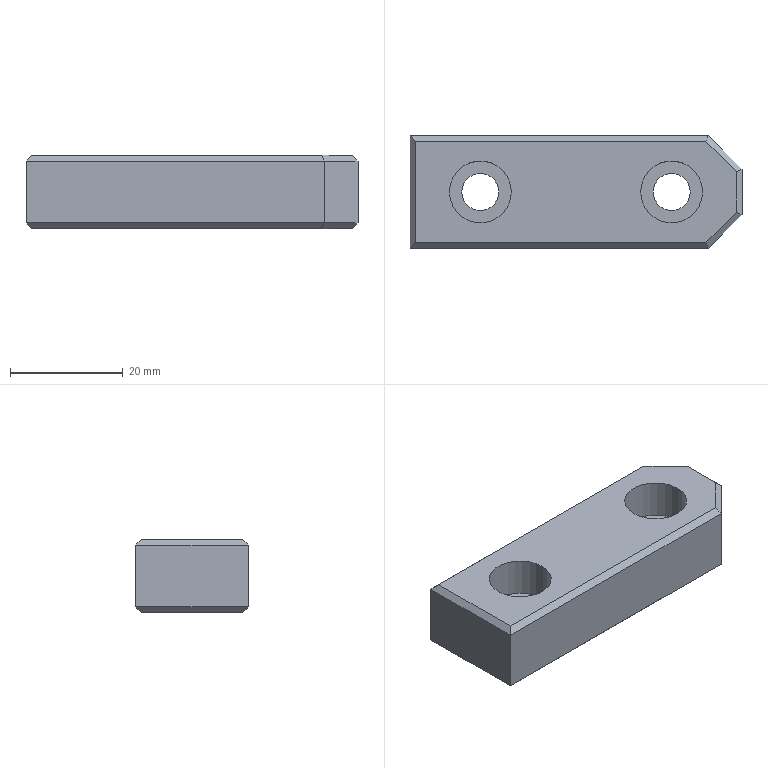Part | Creo | 1 solid | 30 faces | box 59 x 20 x 13 mm | volume 12982 mm3 | plane 22 | cylinder 8 | commonest cylinder face diameters 6.6 x4 11 x4
STEP:
#1=CARTESIAN_POINT('',(0.,0.,0.));
#2=DIRECTION('',(0.,0.,1.));
#3=DIRECTION('',(1.,0.,0.));
#4=AXIS2_PLACEMENT_3D('',#1,#2,#3);
#5=CARTESIAN_POINT('',(-90.,-4.4,-23.828));
#6=VERTEX_POINT('',#5);
#7=CARTESIAN_POINT('',(-90.,-4.4,-34.828));
#8=VERTEX_POINT('',#7);
#9=CARTESIAN_POINT('',(-90.,-4.4,-23.828));
#10=DIRECTION('',(0.,0.,-1.));
#11=VECTOR('',#10,11.);
#12=LINE('',#9,#11);
#13=EDGE_CURVE('',#6,#8,#12,.T.);
#14=ORIENTED_EDGE('',*,*,#13,.F.);
#15=CARTESIAN_POINT('',(-90.,3.6,-23.828));
#16=VERTEX_POINT('',#15);
#17=CARTESIAN_POINT('',(-90.,3.6,-23.828));
#18=DIRECTION('',(0.,-1.,0.));
#19=VECTOR('',#18,8.);
#20=LINE('',#17,#19);
#21=EDGE_CURVE('',#16,#6,#20,.T.);
#22=ORIENTED_EDGE('',*,*,#21,.F.);
#23=CARTESIAN_POINT('',(-90.,3.6,-34.828));
#24=VERTEX_POINT('',#23);
#25=CARTESIAN_POINT('',(-90.,3.6,-34.828));
#26=DIRECTION('',(0.,0.,1.));
#27=VECTOR('',#26,11.);
#28=LINE('',#25,#27);
#29=EDGE_CURVE('',#24,#16,#28,.T.);
#30=ORIENTED_EDGE('',*,*,#29,.F.);
#31=CARTESIAN_POINT('',(-90.,-4.4,-34.828));
#32=DIRECTION('',(0.,1.,0.));
#33=VECTOR('',#32,8.);
#34=LINE('',#31,#33);
#35=EDGE_CURVE('',#8,#24,#34,.T.);
#36=ORIENTED_EDGE('',*,*,#35,.F.);
#37=EDGE_LOOP('',(#14,#22,#30,#36));
#38=FACE_OUTER_BOUND('',#37,.F.);
#39=CARTESIAN_POINT('',(-90.,-10.4,-35.828));
#40=DIRECTION('',(-1.,0.,0.));
#41=DIRECTION('',(0.,0.,-1.));
#42=AXIS2_PLACEMENT_3D('',#39,#40,#41);
#43=PLANE('',#42);
#44=ADVANCED_FACE('',(#38),#43,.F.);
#45=CARTESIAN_POINT('',(-96.,-10.4,-34.828));
#46=VERTEX_POINT('',#45);
#47=CARTESIAN_POINT('',(-96.,-10.4,-23.828));
#48=VERTEX_POINT('',#47);
#49=CARTESIAN_POINT('',(-96.,-10.4,-34.828));
#50=DIRECTION('',(0.,0.,1.));
#51=VECTOR('',#50,11.);
#52=LINE('',#49,#51);
#53=EDGE_CURVE('',#46,#48,#52,.T.);
#54=ORIENTED_EDGE('',*,*,#53,.T.);
#55=CARTESIAN_POINT('',(-90.,-4.4,-23.828));
#56=DIRECTION('',(-0.7071,-0.7071,0.));
#57=VECTOR('',#56,8.485);
#58=LINE('',#55,#57);
#59=EDGE_CURVE('',#6,#48,#58,.T.);
#60=ORIENTED_EDGE('',*,*,#59,.F.);
#61=ORIENTED_EDGE('',*,*,#13,.T.);
#62=CARTESIAN_POINT('',(-96.,-10.4,-34.828));
#63=DIRECTION('',(0.7071,0.7071,0.));
#64=VECTOR('',#63,8.485);
#65=LINE('',#62,#64);
#66=EDGE_CURVE('',#46,#8,#65,.T.);
#67=ORIENTED_EDGE('',*,*,#66,.F.);
#68=EDGE_LOOP('',(#54,#60,#61,#67));
#69=FACE_OUTER_BOUND('',#68,.F.);
#70=CARTESIAN_POINT('',(-96.,-10.4,-35.828));
#71=DIRECTION('',(-0.7071,0.7071,0.));
#72=DIRECTION('',(0.,0.,-1.));
#73=AXIS2_PLACEMENT_3D('',#70,#71,#72);
#74=PLANE('',#73);
#75=ADVANCED_FACE('',(#69),#74,.F.);
#76=ORIENTED_EDGE('',*,*,#53,.F.);
#77=CARTESIAN_POINT('',(-149.,-10.4,-34.828));
#78=VERTEX_POINT('',#77);
#79=CARTESIAN_POINT('',(-149.,-10.4,-34.828));
#80=DIRECTION('',(1.,0.,0.));
#81=VECTOR('',#80,53.);
#82=LINE('',#79,#81);
#83=EDGE_CURVE('',#78,#46,#82,.T.);
#84=ORIENTED_EDGE('',*,*,#83,.F.);
#85=CARTESIAN_POINT('',(-149.,-10.4,-23.828));
#86=VERTEX_POINT('',#85);
#87=CARTESIAN_POINT('',(-149.,-10.4,-23.828));
#88=DIRECTION('',(0.,0.,-1.));
#89=VECTOR('',#88,11.);
#90=LINE('',#87,#89);
#91=EDGE_CURVE('',#86,#78,#90,.T.);
#92=ORIENTED_EDGE('',*,*,#91,.F.);
#93=CARTESIAN_POINT('',(-96.,-10.4,-23.828));
#94=DIRECTION('',(-1.,0.,0.));
#95=VECTOR('',#94,53.);
#96=LINE('',#93,#95);
#97=EDGE_CURVE('',#48,#86,#96,.T.);
#98=ORIENTED_EDGE('',*,*,#97,.F.);
#99=EDGE_LOOP('',(#76,#84,#92,#98));
#100=FACE_OUTER_BOUND('',#99,.F.);
#101=CARTESIAN_POINT('',(-190.,-10.4,-35.828));
#102=DIRECTION('',(0.,1.,0.));
#103=DIRECTION('',(-1.,0.,0.));
#104=AXIS2_PLACEMENT_3D('',#101,#102,#103);
#105=PLANE('',#104);
#106=ADVANCED_FACE('',(#100),#105,.F.);
#107=ORIENTED_EDGE('',*,*,#83,.T.);
#108=CARTESIAN_POINT('',(-96.414,-9.4,-35.828));
#109=VERTEX_POINT('',#108);
#110=CARTESIAN_POINT('',(-96.,-10.4,-34.828));
#111=DIRECTION('',(-0.2811,0.6786,-0.6786));
#112=VECTOR('',#111,1.474);
#113=LINE('',#110,#112);
#114=EDGE_CURVE('',#46,#109,#113,.T.);
#115=ORIENTED_EDGE('',*,*,#114,.T.);
#116=CARTESIAN_POINT('',(-148.,-9.4,-35.828));
#117=VERTEX_POINT('',#116);
#118=CARTESIAN_POINT('',(-96.414,-9.4,-35.828));
#119=DIRECTION('',(-1.,0.,0.));
#120=VECTOR('',#119,51.586);
#121=LINE('',#118,#120);
#122=EDGE_CURVE('',#109,#117,#121,.T.);
#123=ORIENTED_EDGE('',*,*,#122,.T.);
#124=CARTESIAN_POINT('',(-149.,-10.4,-34.828));
#125=DIRECTION('',(0.5774,0.5774,-0.5774));
#126=VECTOR('',#125,1.732);
#127=LINE('',#124,#126);
#128=EDGE_CURVE('',#78,#117,#127,.T.);
#129=ORIENTED_EDGE('',*,*,#128,.F.);
#130=EDGE_LOOP('',(#107,#115,#123,#129));
#131=FACE_OUTER_BOUND('',#130,.F.);
#132=CARTESIAN_POINT('',(-190.,-10.4,-34.828));
#133=DIRECTION('',(0.,-0.7071,-0.7071));
#134=DIRECTION('',(1.,0.,0.));
#135=AXIS2_PLACEMENT_3D('',#132,#133,#134);
#136=PLANE('',#135);
#137=ADVANCED_FACE('',(#131),#136,.T.);
#138=ORIENTED_EDGE('',*,*,#114,.F.);
#139=ORIENTED_EDGE('',*,*,#66,.T.);
#140=CARTESIAN_POINT('',(-91.,-3.986,-35.828));
#141=VERTEX_POINT('',#140);
#142=CARTESIAN_POINT('',(-90.,-4.4,-34.828));
#143=DIRECTION('',(-0.6786,0.2811,-0.6786));
#144=VECTOR('',#143,1.474);
#145=LINE('',#142,#144);
#146=EDGE_CURVE('',#8,#141,#145,.T.);
#147=ORIENTED_EDGE('',*,*,#146,.T.);
#148=CARTESIAN_POINT('',(-91.,-3.986,-35.828));
#149=DIRECTION('',(-0.7071,-0.7071,0.));
#150=VECTOR('',#149,7.657);
#151=LINE('',#148,#150);
#152=EDGE_CURVE('',#141,#109,#151,.T.);
#153=ORIENTED_EDGE('',*,*,#152,.T.);
#154=EDGE_LOOP('',(#138,#139,#147,#153));
#155=FACE_OUTER_BOUND('',#154,.F.);
#156=CARTESIAN_POINT('',(-133.707,-46.693,-35.828));
#157=DIRECTION('',(0.5,-0.5,-0.7071));
#158=DIRECTION('',(-0.7071,-0.7071,0.));
#159=AXIS2_PLACEMENT_3D('',#156,#157,#158);
#160=PLANE('',#159);
#161=ADVANCED_FACE('',(#155),#160,.T.);
#162=ORIENTED_EDGE('',*,*,#146,.F.);
#163=ORIENTED_EDGE('',*,*,#35,.T.);
#164=CARTESIAN_POINT('',(-91.,3.186,-35.828));
#165=VERTEX_POINT('',#164);
#166=CARTESIAN_POINT('',(-90.,3.6,-34.828));
#167=DIRECTION('',(-0.6786,-0.2811,-0.6786));
#168=VECTOR('',#167,1.474);
#169=LINE('',#166,#168);
#170=EDGE_CURVE('',#24,#165,#169,.T.);
#171=ORIENTED_EDGE('',*,*,#170,.T.);
#172=CARTESIAN_POINT('',(-91.,3.186,-35.828));
#173=DIRECTION('',(0.,-1.,0.));
#174=VECTOR('',#173,7.172);
#175=LINE('',#172,#174);
#176=EDGE_CURVE('',#165,#141,#175,.T.);
#177=ORIENTED_EDGE('',*,*,#176,.T.);
#178=EDGE_LOOP('',(#162,#163,#171,#177));
#179=FACE_OUTER_BOUND('',#178,.F.);
#180=CARTESIAN_POINT('',(-90.,-10.4,-34.828));
#181=DIRECTION('',(0.7071,0.,-0.7071));
#182=DIRECTION('',(0.,1.,0.));
#183=AXIS2_PLACEMENT_3D('',#180,#181,#182);
#184=PLANE('',#183);
#185=ADVANCED_FACE('',(#179),#184,.T.);
#186=ORIENTED_EDGE('',*,*,#170,.F.);
#187=CARTESIAN_POINT('',(-96.,9.6,-34.828));
#188=VERTEX_POINT('',#187);
#189=CARTESIAN_POINT('',(-90.,3.6,-34.828));
#190=DIRECTION('',(-0.7071,0.7071,0.));
#191=VECTOR('',#190,8.485);
#192=LINE('',#189,#191);
#193=EDGE_CURVE('',#24,#188,#192,.T.);
#194=ORIENTED_EDGE('',*,*,#193,.T.);
#195=CARTESIAN_POINT('',(-96.414,8.6,-35.828));
#196=VERTEX_POINT('',#195);
#197=CARTESIAN_POINT('',(-96.414,8.6,-35.828));
#198=DIRECTION('',(0.2811,0.6786,0.6786));
#199=VECTOR('',#198,1.474);
#200=LINE('',#197,#199);
#201=EDGE_CURVE('',#196,#188,#200,.T.);
#202=ORIENTED_EDGE('',*,*,#201,.F.);
#203=CARTESIAN_POINT('',(-96.414,8.6,-35.828));
#204=DIRECTION('',(0.7071,-0.7071,0.));
#205=VECTOR('',#204,7.657);
#206=LINE('',#203,#205);
#207=EDGE_CURVE('',#196,#165,#206,.T.);
#208=ORIENTED_EDGE('',*,*,#207,.T.);
#209=EDGE_LOOP('',(#186,#194,#202,#208));
#210=FACE_OUTER_BOUND('',#209,.F.);
#211=CARTESIAN_POINT('',(-143.707,55.893,-35.828));
#212=DIRECTION('',(0.5,0.5,-0.7071));
#213=DIRECTION('',(0.7071,-0.7071,0.));
#214=AXIS2_PLACEMENT_3D('',#211,#212,#213);
#215=PLANE('',#214);
#216=ADVANCED_FACE('',(#210),#215,.T.);
#217=CARTESIAN_POINT('',(-96.,9.6,-23.828));
#218=VERTEX_POINT('',#217);
#219=CARTESIAN_POINT('',(-96.,9.6,-23.828));
#220=DIRECTION('',(0.,0.,-1.));
#221=VECTOR('',#220,11.);
#222=LINE('',#219,#221);
#223=EDGE_CURVE('',#218,#188,#222,.T.);
#224=ORIENTED_EDGE('',*,*,#223,.T.);
#225=ORIENTED_EDGE('',*,*,#193,.F.);
#226=ORIENTED_EDGE('',*,*,#29,.T.);
#227=CARTESIAN_POINT('',(-96.,9.6,-23.828));
#228=DIRECTION('',(0.7071,-0.7071,0.));
#229=VECTOR('',#228,8.485);
#230=LINE('',#227,#229);
#231=EDGE_CURVE('',#218,#16,#230,.T.);
#232=ORIENTED_EDGE('',*,*,#231,.F.);
#233=EDGE_LOOP('',(#224,#225,#226,#232));
#234=FACE_OUTER_BOUND('',#233,.F.);
#235=CARTESIAN_POINT('',(-90.,3.6,-35.828));
#236=DIRECTION('',(-0.7071,-0.7071,0.));
#237=DIRECTION('',(0.,0.,-1.));
#238=AXIS2_PLACEMENT_3D('',#235,#236,#237);
#239=PLANE('',#238);
#240=ADVANCED_FACE('',(#234),#239,.F.);
#241=ORIENTED_EDGE('',*,*,#223,.F.);
#242=CARTESIAN_POINT('',(-149.,9.6,-23.828));
#243=VERTEX_POINT('',#242);
#244=CARTESIAN_POINT('',(-149.,9.6,-23.828));
#245=DIRECTION('',(1.,0.,0.));
#246=VECTOR('',#245,53.);
#247=LINE('',#244,#246);
#248=EDGE_CURVE('',#243,#218,#247,.T.);
#249=ORIENTED_EDGE('',*,*,#248,.F.);
#250=CARTESIAN_POINT('',(-149.,9.6,-34.828));
#251=VERTEX_POINT('',#250);
#252=CARTESIAN_POINT('',(-149.,9.6,-23.828));
#253=DIRECTION('',(0.,0.,-1.));
#254=VECTOR('',#253,11.);
#255=LINE('',#252,#254);
#256=EDGE_CURVE('',#243,#251,#255,.T.);
#257=ORIENTED_EDGE('',*,*,#256,.T.);
#258=CARTESIAN_POINT('',(-96.,9.6,-34.828));
#259=DIRECTION('',(-1.,0.,0.));
#260=VECTOR('',#259,53.);
#261=LINE('',#258,#260);
#262=EDGE_CURVE('',#188,#251,#261,.T.);
#263=ORIENTED_EDGE('',*,*,#262,.F.);
#264=EDGE_LOOP('',(#241,#249,#257,#263));
#265=FACE_OUTER_BOUND('',#264,.F.);
#266=CARTESIAN_POINT('',(-90.,9.6,-35.828));
#267=DIRECTION('',(0.,-1.,0.));
#268=DIRECTION('',(1.,0.,0.));
#269=AXIS2_PLACEMENT_3D('',#266,#267,#268);
#270=PLANE('',#269);
#271=ADVANCED_FACE('',(#265),#270,.F.);
#272=CARTESIAN_POINT('',(-96.414,8.6,-22.828));
#273=VERTEX_POINT('',#272);
#274=CARTESIAN_POINT('',(-96.414,8.6,-22.828));
#275=DIRECTION('',(0.2811,0.6786,-0.6786));
#276=VECTOR('',#275,1.474);
#277=LINE('',#274,#276);
#278=EDGE_CURVE('',#273,#218,#277,.T.);
#279=ORIENTED_EDGE('',*,*,#278,.F.);
#280=CARTESIAN_POINT('',(-148.,8.6,-22.828));
#281=VERTEX_POINT('',#280);
#282=CARTESIAN_POINT('',(-96.414,8.6,-22.828));
#283=DIRECTION('',(-1.,0.,0.));
#284=VECTOR('',#283,51.586);
#285=LINE('',#282,#284);
#286=EDGE_CURVE('',#273,#281,#285,.T.);
#287=ORIENTED_EDGE('',*,*,#286,.T.);
#288=CARTESIAN_POINT('',(-149.,9.6,-23.828));
#289=DIRECTION('',(0.5774,-0.5774,0.5774));
#290=VECTOR('',#289,1.732);
#291=LINE('',#288,#290);
#292=EDGE_CURVE('',#243,#281,#291,.T.);
#293=ORIENTED_EDGE('',*,*,#292,.F.);
#294=ORIENTED_EDGE('',*,*,#248,.T.);
#295=EDGE_LOOP('',(#279,#287,#293,#294));
#296=FACE_OUTER_BOUND('',#295,.F.);
#297=CARTESIAN_POINT('',(-90.,9.6,-23.828));
#298=DIRECTION('',(0.,-0.7071,-0.7071));
#299=DIRECTION('',(-1.,0.,0.));
#300=AXIS2_PLACEMENT_3D('',#297,#298,#299);
#301=PLANE('',#300);
#302=ADVANCED_FACE('',(#296),#301,.F.);
#303=CARTESIAN_POINT('',(-91.,3.186,-22.828));
#304=VERTEX_POINT('',#303);
#305=CARTESIAN_POINT('',(-91.,3.186,-22.828));
#306=DIRECTION('',(0.6786,0.2811,-0.6786));
#307=VECTOR('',#306,1.474);
#308=LINE('',#305,#307);
#309=EDGE_CURVE('',#304,#16,#308,.T.);
#310=ORIENTED_EDGE('',*,*,#309,.F.);
#311=CARTESIAN_POINT('',(-91.,3.186,-22.828));
#312=DIRECTION('',(-0.7071,0.7071,0.));
#313=VECTOR('',#312,7.657);
#314=LINE('',#311,#313);
#315=EDGE_CURVE('',#304,#273,#314,.T.);
#316=ORIENTED_EDGE('',*,*,#315,.T.);
#317=ORIENTED_EDGE('',*,*,#278,.T.);
#318=ORIENTED_EDGE('',*,*,#231,.T.);
#319=EDGE_LOOP('',(#310,#316,#317,#318));
#320=FACE_OUTER_BOUND('',#319,.F.);
#321=CARTESIAN_POINT('',(-143.707,55.893,-22.828));
#322=DIRECTION('',(-0.5,-0.5,-0.7071));
#323=DIRECTION('',(0.7071,-0.7071,0.));
#324=AXIS2_PLACEMENT_3D('',#321,#322,#323);
#325=PLANE('',#324);
#326=ADVANCED_FACE('',(#320),#325,.F.);
#327=CARTESIAN_POINT('',(-91.,-3.986,-22.828));
#328=VERTEX_POINT('',#327);
#329=CARTESIAN_POINT('',(-91.,-3.986,-22.828));
#330=DIRECTION('',(0.6786,-0.2811,-0.6786));
#331=VECTOR('',#330,1.474);
#332=LINE('',#329,#331);
#333=EDGE_CURVE('',#328,#6,#332,.T.);
#334=ORIENTED_EDGE('',*,*,#333,.F.);
#335=CARTESIAN_POINT('',(-91.,-3.986,-22.828));
#336=DIRECTION('',(0.,1.,0.));
#337=VECTOR('',#336,7.172);
#338=LINE('',#335,#337);
#339=EDGE_CURVE('',#328,#304,#338,.T.);
#340=ORIENTED_EDGE('',*,*,#339,.T.);
#341=ORIENTED_EDGE('',*,*,#309,.T.);
#342=ORIENTED_EDGE('',*,*,#21,.T.);
#343=EDGE_LOOP('',(#334,#340,#341,#342));
#344=FACE_OUTER_BOUND('',#343,.F.);
#345=CARTESIAN_POINT('',(-91.,9.6,-22.828));
#346=DIRECTION('',(-0.7071,0.,-0.7071));
#347=DIRECTION('',(0.,-1.,0.));
#348=AXIS2_PLACEMENT_3D('',#345,#346,#347);
#349=PLANE('',#348);
#350=ADVANCED_FACE('',(#344),#349,.F.);
#351=CARTESIAN_POINT('',(-96.414,-9.4,-22.828));
#352=VERTEX_POINT('',#351);
#353=CARTESIAN_POINT('',(-96.414,-9.4,-22.828));
#354=DIRECTION('',(0.2811,-0.6786,-0.6786));
#355=VECTOR('',#354,1.474);
#356=LINE('',#353,#355);
#357=EDGE_CURVE('',#352,#48,#356,.T.);
#358=ORIENTED_EDGE('',*,*,#357,.F.);
#359=CARTESIAN_POINT('',(-96.414,-9.4,-22.828));
#360=DIRECTION('',(0.7071,0.7071,0.));
#361=VECTOR('',#360,7.657);
#362=LINE('',#359,#361);
#363=EDGE_CURVE('',#352,#328,#362,.T.);
#364=ORIENTED_EDGE('',*,*,#363,.T.);
#365=ORIENTED_EDGE('',*,*,#333,.T.);
#366=ORIENTED_EDGE('',*,*,#59,.T.);
#367=EDGE_LOOP('',(#358,#364,#365,#366));
#368=FACE_OUTER_BOUND('',#367,.F.);
#369=CARTESIAN_POINT('',(-133.707,-46.693,-22.828));
#370=DIRECTION('',(-0.5,0.5,-0.7071));
#371=DIRECTION('',(-0.7071,-0.7071,0.));
#372=AXIS2_PLACEMENT_3D('',#369,#370,#371);
#373=PLANE('',#372);
#374=ADVANCED_FACE('',(#368),#373,.F.);
#375=CARTESIAN_POINT('',(-148.,-9.4,-22.828));
#376=VERTEX_POINT('',#375);
#377=CARTESIAN_POINT('',(-148.,-9.4,-22.828));
#378=DIRECTION('',(1.,0.,0.));
#379=VECTOR('',#378,51.586);
#380=LINE('',#377,#379);
#381=EDGE_CURVE('',#376,#352,#380,.T.);
#382=ORIENTED_EDGE('',*,*,#381,.T.);
#383=ORIENTED_EDGE('',*,*,#357,.T.);
#384=ORIENTED_EDGE('',*,*,#97,.T.);
#385=CARTESIAN_POINT('',(-149.,-10.4,-23.828));
#386=DIRECTION('',(0.5774,0.5774,0.5774));
#387=VECTOR('',#386,1.732);
#388=LINE('',#385,#387);
#389=EDGE_CURVE('',#86,#376,#388,.T.);
#390=ORIENTED_EDGE('',*,*,#389,.T.);
#391=EDGE_LOOP('',(#382,#383,#384,#390));
#392=FACE_OUTER_BOUND('',#391,.F.);
#393=CARTESIAN_POINT('',(-190.,-9.4,-22.828));
#394=DIRECTION('',(0.,0.7071,-0.7071));
#395=DIRECTION('',(-1.,0.,0.));
#396=AXIS2_PLACEMENT_3D('',#393,#394,#395);
#397=PLANE('',#396);
#398=ADVANCED_FACE('',(#392),#397,.F.);
#399=ORIENTED_EDGE('',*,*,#315,.F.);
#400=ORIENTED_EDGE('',*,*,#339,.F.);
#401=ORIENTED_EDGE('',*,*,#363,.F.);
#402=ORIENTED_EDGE('',*,*,#381,.F.);
#403=CARTESIAN_POINT('',(-148.,8.6,-22.828));
#404=DIRECTION('',(0.,-1.,0.));
#405=VECTOR('',#404,18.);
#406=LINE('',#403,#405);
#407=EDGE_CURVE('',#281,#376,#406,.T.);
#408=ORIENTED_EDGE('',*,*,#407,.F.);
#409=ORIENTED_EDGE('',*,*,#286,.F.);
#410=EDGE_LOOP('',(#399,#400,#401,#402,#408,#409));
#411=FACE_OUTER_BOUND('',#410,.F.);
#412=CARTESIAN_POINT('',(-142.,-0.4,-22.828));
#413=VERTEX_POINT('',#412);
#414=CARTESIAN_POINT('',(-131.,-0.4,-22.828));
#415=VERTEX_POINT('',#414);
#416=CARTESIAN_POINT('',(-136.5,-0.4,-22.828));
#417=DIRECTION('',(0.,0.,-1.));
#418=DIRECTION('',(-1.,0.,0.));
#419=AXIS2_PLACEMENT_3D('',#416,#417,#418);
#420=CIRCLE('',#419,5.5);
#421=EDGE_CURVE('',#413,#415,#420,.T.);
#422=ORIENTED_EDGE('',*,*,#421,.F.);
#423=CARTESIAN_POINT('',(-136.5,-0.4,-22.828));
#424=DIRECTION('',(0.,0.,-1.));
#425=DIRECTION('',(1.,0.,0.));
#426=AXIS2_PLACEMENT_3D('',#423,#424,#425);
#427=CIRCLE('',#426,5.5);
#428=EDGE_CURVE('',#415,#413,#427,.T.);
#429=ORIENTED_EDGE('',*,*,#428,.F.);
#430=EDGE_LOOP('',(#422,#429));
#431=FACE_BOUND('',#430,.F.);
#432=CARTESIAN_POINT('',(-108.,-0.4,-22.828));
#433=VERTEX_POINT('',#432);
#434=CARTESIAN_POINT('',(-97.,-0.4,-22.828));
#435=VERTEX_POINT('',#434);
#436=CARTESIAN_POINT('',(-102.5,-0.4,-22.828));
#437=DIRECTION('',(0.,0.,-1.));
#438=DIRECTION('',(-1.,0.,0.));
#439=AXIS2_PLACEMENT_3D('',#436,#437,#438);
#440=CIRCLE('',#439,5.5);
#441=EDGE_CURVE('',#433,#435,#440,.T.);
#442=ORIENTED_EDGE('',*,*,#441,.F.);
#443=CARTESIAN_POINT('',(-102.5,-0.4,-22.828));
#444=DIRECTION('',(0.,0.,-1.));
#445=DIRECTION('',(1.,0.,0.));
#446=AXIS2_PLACEMENT_3D('',#443,#444,#445);
#447=CIRCLE('',#446,5.5);
#448=EDGE_CURVE('',#435,#433,#447,.T.);
#449=ORIENTED_EDGE('',*,*,#448,.F.);
#450=EDGE_LOOP('',(#442,#449));
#451=FACE_BOUND('',#450,.F.);
#452=CARTESIAN_POINT('',(-190.,9.6,-22.828));
#453=DIRECTION('',(0.,0.,-1.));
#454=DIRECTION('',(0.,-1.,0.));
#455=AXIS2_PLACEMENT_3D('',#452,#453,#454);
#456=PLANE('',#455);
#457=ADVANCED_FACE('',(#411,#431,#451),#456,.F.);
#458=CARTESIAN_POINT('',(-149.,-10.4,-23.828));
#459=DIRECTION('',(0.,1.,0.));
#460=VECTOR('',#459,20.);
#461=LINE('',#458,#460);
#462=EDGE_CURVE('',#86,#243,#461,.T.);
#463=ORIENTED_EDGE('',*,*,#462,.T.);
#464=ORIENTED_EDGE('',*,*,#292,.T.);
#465=ORIENTED_EDGE('',*,*,#407,.T.);
#466=ORIENTED_EDGE('',*,*,#389,.F.);
#467=EDGE_LOOP('',(#463,#464,#465,#466));
#468=FACE_OUTER_BOUND('',#467,.F.);
#469=CARTESIAN_POINT('',(-149.,-0.4,-23.828));
#470=DIRECTION('',(0.7071,0.,-0.7071));
#471=DIRECTION('',(0.,-1.,0.));
#472=AXIS2_PLACEMENT_3D('',#469,#470,#471);
#473=PLANE('',#472);
#474=ADVANCED_FACE('',(#468),#473,.F.);
#475=CARTESIAN_POINT('',(-149.,9.6,-34.828));
#476=DIRECTION('',(0.,-1.,0.));
#477=VECTOR('',#476,20.);
#478=LINE('',#475,#477);
#479=EDGE_CURVE('',#251,#78,#478,.T.);
#480=ORIENTED_EDGE('',*,*,#479,.F.);
#481=ORIENTED_EDGE('',*,*,#256,.F.);
#482=ORIENTED_EDGE('',*,*,#462,.F.);
#483=ORIENTED_EDGE('',*,*,#91,.T.);
#484=EDGE_LOOP('',(#480,#481,#482,#483));
#485=FACE_OUTER_BOUND('',#484,.F.);
#486=CARTESIAN_POINT('',(-149.,-0.4,17.172));
#487=DIRECTION('',(1.,0.,0.));
#488=DIRECTION('',(0.,0.,-1.));
#489=AXIS2_PLACEMENT_3D('',#486,#487,#488);
#490=PLANE('',#489);
#491=ADVANCED_FACE('',(#485),#490,.F.);
#492=CARTESIAN_POINT('',(-148.,8.6,-35.828));
#493=VERTEX_POINT('',#492);
#494=CARTESIAN_POINT('',(-148.,-9.4,-35.828));
#495=DIRECTION('',(0.,1.,0.));
#496=VECTOR('',#495,18.);
#497=LINE('',#494,#496);
#498=EDGE_CURVE('',#117,#493,#497,.T.);
#499=ORIENTED_EDGE('',*,*,#498,.T.);
#500=CARTESIAN_POINT('',(-149.,9.6,-34.828));
#501=DIRECTION('',(0.5774,-0.5774,-0.5774));
#502=VECTOR('',#501,1.732);
#503=LINE('',#500,#502);
#504=EDGE_CURVE('',#251,#493,#503,.T.);
#505=ORIENTED_EDGE('',*,*,#504,.F.);
#506=ORIENTED_EDGE('',*,*,#479,.T.);
#507=ORIENTED_EDGE('',*,*,#128,.T.);
#508=EDGE_LOOP('',(#499,#505,#506,#507));
#509=FACE_OUTER_BOUND('',#508,.F.);
#510=CARTESIAN_POINT('',(-149.,-0.4,-34.828));
#511=DIRECTION('',(-0.7071,0.,-0.7071));
#512=DIRECTION('',(0.,-1.,0.));
#513=AXIS2_PLACEMENT_3D('',#510,#511,#512);
#514=PLANE('',#513);
#515=ADVANCED_FACE('',(#509),#514,.T.);
#516=ORIENTED_EDGE('',*,*,#498,.F.);
#517=ORIENTED_EDGE('',*,*,#122,.F.);
#518=ORIENTED_EDGE('',*,*,#152,.F.);
#519=ORIENTED_EDGE('',*,*,#176,.F.);
#520=ORIENTED_EDGE('',*,*,#207,.F.);
#521=CARTESIAN_POINT('',(-148.,8.6,-35.828));
#522=DIRECTION('',(1.,0.,0.));
#523=VECTOR('',#522,51.586);
#524=LINE('',#521,#523);
#525=EDGE_CURVE('',#493,#196,#524,.T.);
#526=ORIENTED_EDGE('',*,*,#525,.F.);
#527=EDGE_LOOP('',(#516,#517,#518,#519,#520,#526));
#528=FACE_OUTER_BOUND('',#527,.F.);
#529=CARTESIAN_POINT('',(-139.8,-0.4,-35.828));
#530=VERTEX_POINT('',#529);
#531=CARTESIAN_POINT('',(-133.2,-0.4,-35.828));
#532=VERTEX_POINT('',#531);
#533=CARTESIAN_POINT('',(-136.5,-0.4,-35.828));
#534=DIRECTION('',(0.,0.,1.));
#535=DIRECTION('',(-1.,0.,0.));
#536=AXIS2_PLACEMENT_3D('',#533,#534,#535);
#537=CIRCLE('',#536,3.3);
#538=EDGE_CURVE('',#530,#532,#537,.T.);
#539=ORIENTED_EDGE('',*,*,#538,.F.);
#540=CARTESIAN_POINT('',(-136.5,-0.4,-35.828));
#541=DIRECTION('',(0.,0.,1.));
#542=DIRECTION('',(1.,0.,0.));
#543=AXIS2_PLACEMENT_3D('',#540,#541,#542);
#544=CIRCLE('',#543,3.3);
#545=EDGE_CURVE('',#532,#530,#544,.T.);
#546=ORIENTED_EDGE('',*,*,#545,.F.);
#547=EDGE_LOOP('',(#539,#546));
#548=FACE_BOUND('',#547,.F.);
#549=CARTESIAN_POINT('',(-105.8,-0.4,-35.828));
#550=VERTEX_POINT('',#549);
#551=CARTESIAN_POINT('',(-99.2,-0.4,-35.828));
#552=VERTEX_POINT('',#551);
#553=CARTESIAN_POINT('',(-102.5,-0.4,-35.828));
#554=DIRECTION('',(0.,0.,1.));
#555=DIRECTION('',(-1.,0.,0.));
#556=AXIS2_PLACEMENT_3D('',#553,#554,#555);
#557=CIRCLE('',#556,3.3);
#558=EDGE_CURVE('',#550,#552,#557,.T.);
#559=ORIENTED_EDGE('',*,*,#558,.F.);
#560=CARTESIAN_POINT('',(-102.5,-0.4,-35.828));
#561=DIRECTION('',(0.,0.,1.));
#562=DIRECTION('',(1.,0.,0.));
#563=AXIS2_PLACEMENT_3D('',#560,#561,#562);
#564=CIRCLE('',#563,3.3);
#565=EDGE_CURVE('',#552,#550,#564,.T.);
#566=ORIENTED_EDGE('',*,*,#565,.F.);
#567=EDGE_LOOP('',(#559,#566));
#568=FACE_BOUND('',#567,.F.);
#569=CARTESIAN_POINT('',(-190.,9.6,-35.828));
#570=DIRECTION('',(0.,0.,-1.));
#571=DIRECTION('',(0.,-1.,0.));
#572=AXIS2_PLACEMENT_3D('',#569,#570,#571);
#573=PLANE('',#572);
#574=ADVANCED_FACE('',(#528,#548,#568),#573,.T.);
#575=ORIENTED_EDGE('',*,*,#525,.T.);
#576=ORIENTED_EDGE('',*,*,#201,.T.);
#577=ORIENTED_EDGE('',*,*,#262,.T.);
#578=ORIENTED_EDGE('',*,*,#504,.T.);
#579=EDGE_LOOP('',(#575,#576,#577,#578));
#580=FACE_OUTER_BOUND('',#579,.F.);
#581=CARTESIAN_POINT('',(-190.,8.6,-35.828));
#582=DIRECTION('',(0.,0.7071,-0.7071));
#583=DIRECTION('',(1.,0.,0.));
#584=AXIS2_PLACEMENT_3D('',#581,#582,#583);
#585=PLANE('',#584);
#586=ADVANCED_FACE('',(#580),#585,.T.);
#587=CARTESIAN_POINT('',(-133.2,-0.4,-29.828));
#588=VERTEX_POINT('',#587);
#589=CARTESIAN_POINT('',(-139.8,-0.4,-29.828));
#590=VERTEX_POINT('',#589);
#591=CARTESIAN_POINT('',(-136.5,-0.4,-29.828));
#592=DIRECTION('',(0.,0.,-1.));
#593=DIRECTION('',(1.,0.,0.));
#594=AXIS2_PLACEMENT_3D('',#591,#592,#593);
#595=CIRCLE('',#594,3.3);
#596=EDGE_CURVE('',#588,#590,#595,.T.);
#597=ORIENTED_EDGE('',*,*,#596,.T.);
#598=CARTESIAN_POINT('',(-139.8,-0.4,-29.828));
#599=DIRECTION('',(0.,0.,-1.));
#600=VECTOR('',#599,6.);
#601=LINE('',#598,#600);
#602=EDGE_CURVE('',#590,#530,#601,.T.);
#603=ORIENTED_EDGE('',*,*,#602,.T.);
#604=ORIENTED_EDGE('',*,*,#538,.T.);
#605=CARTESIAN_POINT('',(-133.2,-0.4,-29.828));
#606=DIRECTION('',(0.,0.,-1.));
#607=VECTOR('',#606,6.);
#608=LINE('',#605,#607);
#609=EDGE_CURVE('',#588,#532,#608,.T.);
#610=ORIENTED_EDGE('',*,*,#609,.F.);
#611=EDGE_LOOP('',(#597,#603,#604,#610));
#612=FACE_OUTER_BOUND('',#611,.F.);
#613=CARTESIAN_POINT('',(-136.5,-0.4,-222.827));
#614=DIRECTION('',(0.,0.,-1.));
#615=DIRECTION('',(-1.,0.,0.));
#616=AXIS2_PLACEMENT_3D('',#613,#614,#615);
#617=CYLINDRICAL_SURFACE('',#616,3.3);
#618=ADVANCED_FACE('',(#612),#617,.F.);
#619=CARTESIAN_POINT('',(-142.,-0.4,-29.828));
#620=VERTEX_POINT('',#619);
#621=CARTESIAN_POINT('',(-131.,-0.4,-29.828));
#622=VERTEX_POINT('',#621);
#623=CARTESIAN_POINT('',(-136.5,-0.4,-29.828));
#624=DIRECTION('',(0.,0.,1.));
#625=DIRECTION('',(-1.,0.,0.));
#626=AXIS2_PLACEMENT_3D('',#623,#624,#625);
#627=CIRCLE('',#626,5.5);
#628=EDGE_CURVE('',#620,#622,#627,.T.);
#629=ORIENTED_EDGE('',*,*,#628,.F.);
#630=CARTESIAN_POINT('',(-136.5,-0.4,-29.828));
#631=DIRECTION('',(0.,0.,1.));
#632=DIRECTION('',(1.,0.,0.));
#633=AXIS2_PLACEMENT_3D('',#630,#631,#632);
#634=CIRCLE('',#633,5.5);
#635=EDGE_CURVE('',#622,#620,#634,.T.);
#636=ORIENTED_EDGE('',*,*,#635,.F.);
#637=EDGE_LOOP('',(#629,#636));
#638=FACE_OUTER_BOUND('',#637,.F.);
#639=CARTESIAN_POINT('',(-136.5,-0.4,-29.828));
#640=DIRECTION('',(0.,0.,-1.));
#641=DIRECTION('',(-1.,0.,0.));
#642=AXIS2_PLACEMENT_3D('',#639,#640,#641);
#643=CIRCLE('',#642,3.3);
#644=EDGE_CURVE('',#590,#588,#643,.T.);
#645=ORIENTED_EDGE('',*,*,#644,.F.);
#646=ORIENTED_EDGE('',*,*,#596,.F.);
#647=EDGE_LOOP('',(#645,#646));
#648=FACE_BOUND('',#647,.F.);
#649=CARTESIAN_POINT('',(-136.5,-5.9,-29.828));
#650=DIRECTION('',(0.,0.,-1.));
#651=DIRECTION('',(1.,0.,0.));
#652=AXIS2_PLACEMENT_3D('',#649,#650,#651);
#653=PLANE('',#652);
#654=ADVANCED_FACE('',(#638,#648),#653,.F.);
#655=ORIENTED_EDGE('',*,*,#644,.T.);
#656=ORIENTED_EDGE('',*,*,#609,.T.);
#657=ORIENTED_EDGE('',*,*,#545,.T.);
#658=ORIENTED_EDGE('',*,*,#602,.F.);
#659=EDGE_LOOP('',(#655,#656,#657,#658));
#660=FACE_OUTER_BOUND('',#659,.F.);
#661=CARTESIAN_POINT('',(-136.5,-0.4,-222.827));
#662=DIRECTION('',(0.,0.,-1.));
#663=DIRECTION('',(-1.,0.,0.));
#664=AXIS2_PLACEMENT_3D('',#661,#662,#663);
#665=CYLINDRICAL_SURFACE('',#664,3.3);
#666=ADVANCED_FACE('',(#660),#665,.F.);
#667=ORIENTED_EDGE('',*,*,#428,.T.);
#668=CARTESIAN_POINT('',(-142.,-0.4,-22.828));
#669=DIRECTION('',(0.,0.,-1.));
#670=VECTOR('',#669,7.);
#671=LINE('',#668,#670);
#672=EDGE_CURVE('',#413,#620,#671,.T.);
#673=ORIENTED_EDGE('',*,*,#672,.T.);
#674=ORIENTED_EDGE('',*,*,#628,.T.);
#675=CARTESIAN_POINT('',(-131.,-0.4,-22.828));
#676=DIRECTION('',(0.,0.,-1.));
#677=VECTOR('',#676,7.);
#678=LINE('',#675,#677);
#679=EDGE_CURVE('',#415,#622,#678,.T.);
#680=ORIENTED_EDGE('',*,*,#679,.F.);
#681=EDGE_LOOP('',(#667,#673,#674,#680));
#682=FACE_OUTER_BOUND('',#681,.F.);
#683=CARTESIAN_POINT('',(-136.5,-0.4,-22.828));
#684=DIRECTION('',(0.,0.,-1.));
#685=DIRECTION('',(-1.,0.,0.));
#686=AXIS2_PLACEMENT_3D('',#683,#684,#685);
#687=CYLINDRICAL_SURFACE('',#686,5.5);
#688=ADVANCED_FACE('',(#682),#687,.F.);
#689=ORIENTED_EDGE('',*,*,#421,.T.);
#690=ORIENTED_EDGE('',*,*,#679,.T.);
#691=ORIENTED_EDGE('',*,*,#635,.T.);
#692=ORIENTED_EDGE('',*,*,#672,.F.);
#693=EDGE_LOOP('',(#689,#690,#691,#692));
#694=FACE_OUTER_BOUND('',#693,.F.);
#695=CARTESIAN_POINT('',(-136.5,-0.4,-22.828));
#696=DIRECTION('',(0.,0.,-1.));
#697=DIRECTION('',(-1.,0.,0.));
#698=AXIS2_PLACEMENT_3D('',#695,#696,#697);
#699=CYLINDRICAL_SURFACE('',#698,5.5);
#700=ADVANCED_FACE('',(#694),#699,.F.);
#701=CARTESIAN_POINT('',(-99.2,-0.4,-29.828));
#702=VERTEX_POINT('',#701);
#703=CARTESIAN_POINT('',(-105.8,-0.4,-29.828));
#704=VERTEX_POINT('',#703);
#705=CARTESIAN_POINT('',(-102.5,-0.4,-29.828));
#706=DIRECTION('',(0.,0.,-1.));
#707=DIRECTION('',(1.,0.,0.));
#708=AXIS2_PLACEMENT_3D('',#705,#706,#707);
#709=CIRCLE('',#708,3.3);
#710=EDGE_CURVE('',#702,#704,#709,.T.);
#711=ORIENTED_EDGE('',*,*,#710,.T.);
#712=CARTESIAN_POINT('',(-105.8,-0.4,-29.828));
#713=DIRECTION('',(0.,0.,-1.));
#714=VECTOR('',#713,6.);
#715=LINE('',#712,#714);
#716=EDGE_CURVE('',#704,#550,#715,.T.);
#717=ORIENTED_EDGE('',*,*,#716,.T.);
#718=ORIENTED_EDGE('',*,*,#558,.T.);
#719=CARTESIAN_POINT('',(-99.2,-0.4,-29.828));
#720=DIRECTION('',(0.,0.,-1.));
#721=VECTOR('',#720,6.);
#722=LINE('',#719,#721);
#723=EDGE_CURVE('',#702,#552,#722,.T.);
#724=ORIENTED_EDGE('',*,*,#723,.F.);
#725=EDGE_LOOP('',(#711,#717,#718,#724));
#726=FACE_OUTER_BOUND('',#725,.F.);
#727=CARTESIAN_POINT('',(-102.5,-0.4,-222.827));
#728=DIRECTION('',(0.,0.,-1.));
#729=DIRECTION('',(-1.,0.,0.));
#730=AXIS2_PLACEMENT_3D('',#727,#728,#729);
#731=CYLINDRICAL_SURFACE('',#730,3.3);
#732=ADVANCED_FACE('',(#726),#731,.F.);
#733=CARTESIAN_POINT('',(-108.,-0.4,-29.828));
#734=VERTEX_POINT('',#733);
#735=CARTESIAN_POINT('',(-97.,-0.4,-29.828));
#736=VERTEX_POINT('',#735);
#737=CARTESIAN_POINT('',(-102.5,-0.4,-29.828));
#738=DIRECTION('',(0.,0.,1.));
#739=DIRECTION('',(-1.,0.,0.));
#740=AXIS2_PLACEMENT_3D('',#737,#738,#739);
#741=CIRCLE('',#740,5.5);
#742=EDGE_CURVE('',#734,#736,#741,.T.);
#743=ORIENTED_EDGE('',*,*,#742,.F.);
#744=CARTESIAN_POINT('',(-102.5,-0.4,-29.828));
#745=DIRECTION('',(0.,0.,1.));
#746=DIRECTION('',(1.,0.,0.));
#747=AXIS2_PLACEMENT_3D('',#744,#745,#746);
#748=CIRCLE('',#747,5.5);
#749=EDGE_CURVE('',#736,#734,#748,.T.);
#750=ORIENTED_EDGE('',*,*,#749,.F.);
#751=EDGE_LOOP('',(#743,#750));
#752=FACE_OUTER_BOUND('',#751,.F.);
#753=CARTESIAN_POINT('',(-102.5,-0.4,-29.828));
#754=DIRECTION('',(0.,0.,-1.));
#755=DIRECTION('',(-1.,0.,0.));
#756=AXIS2_PLACEMENT_3D('',#753,#754,#755);
#757=CIRCLE('',#756,3.3);
#758=EDGE_CURVE('',#704,#702,#757,.T.);
#759=ORIENTED_EDGE('',*,*,#758,.F.);
#760=ORIENTED_EDGE('',*,*,#710,.F.);
#761=EDGE_LOOP('',(#759,#760));
#762=FACE_BOUND('',#761,.F.);
#763=CARTESIAN_POINT('',(-102.5,-5.9,-29.828));
#764=DIRECTION('',(0.,0.,-1.));
#765=DIRECTION('',(1.,0.,0.));
#766=AXIS2_PLACEMENT_3D('',#763,#764,#765);
#767=PLANE('',#766);
#768=ADVANCED_FACE('',(#752,#762),#767,.F.);
#769=ORIENTED_EDGE('',*,*,#758,.T.);
#770=ORIENTED_EDGE('',*,*,#723,.T.);
#771=ORIENTED_EDGE('',*,*,#565,.T.);
#772=ORIENTED_EDGE('',*,*,#716,.F.);
#773=EDGE_LOOP('',(#769,#770,#771,#772));
#774=FACE_OUTER_BOUND('',#773,.F.);
#775=CARTESIAN_POINT('',(-102.5,-0.4,-222.827));
#776=DIRECTION('',(0.,0.,-1.));
#777=DIRECTION('',(-1.,0.,0.));
#778=AXIS2_PLACEMENT_3D('',#775,#776,#777);
#779=CYLINDRICAL_SURFACE('',#778,3.3);
#780=ADVANCED_FACE('',(#774),#779,.F.);
#781=ORIENTED_EDGE('',*,*,#448,.T.);
#782=CARTESIAN_POINT('',(-108.,-0.4,-22.828));
#783=DIRECTION('',(0.,0.,-1.));
#784=VECTOR('',#783,7.);
#785=LINE('',#782,#784);
#786=EDGE_CURVE('',#433,#734,#785,.T.);
#787=ORIENTED_EDGE('',*,*,#786,.T.);
#788=ORIENTED_EDGE('',*,*,#742,.T.);
#789=CARTESIAN_POINT('',(-97.,-0.4,-22.828));
#790=DIRECTION('',(0.,0.,-1.));
#791=VECTOR('',#790,7.);
#792=LINE('',#789,#791);
#793=EDGE_CURVE('',#435,#736,#792,.T.);
#794=ORIENTED_EDGE('',*,*,#793,.F.);
#795=EDGE_LOOP('',(#781,#787,#788,#794));
#796=FACE_OUTER_BOUND('',#795,.F.);
#797=CARTESIAN_POINT('',(-102.5,-0.4,-22.828));
#798=DIRECTION('',(0.,0.,-1.));
#799=DIRECTION('',(-1.,0.,0.));
#800=AXIS2_PLACEMENT_3D('',#797,#798,#799);
#801=CYLINDRICAL_SURFACE('',#800,5.5);
#802=ADVANCED_FACE('',(#796),#801,.F.);
#803=ORIENTED_EDGE('',*,*,#441,.T.);
#804=ORIENTED_EDGE('',*,*,#793,.T.);
#805=ORIENTED_EDGE('',*,*,#749,.T.);
#806=ORIENTED_EDGE('',*,*,#786,.F.);
#807=EDGE_LOOP('',(#803,#804,#805,#806));
#808=FACE_OUTER_BOUND('',#807,.F.);
#809=CARTESIAN_POINT('',(-102.5,-0.4,-22.828));
#810=DIRECTION('',(0.,0.,-1.));
#811=DIRECTION('',(-1.,0.,0.));
#812=AXIS2_PLACEMENT_3D('',#809,#810,#811);
#813=CYLINDRICAL_SURFACE('',#812,5.5);
#814=ADVANCED_FACE('',(#808),#813,.F.);
#815=CLOSED_SHELL('',(#44,#75,#106,#137,#161,#185,#216,#240,#271,#302,#326,#350,#374,#398,#457,#474,#491,#515,#574,#586,#618,#654,#666,#688,#700,#732,#768,#780,#802,#814));
#816=MANIFOLD_SOLID_BREP('',#815);
#817=(LENGTH_UNIT()NAMED_UNIT(*)SI_UNIT(.MILLI.,.METRE.));
#818=UNCERTAINTY_MEASURE_WITH_UNIT(LENGTH_MEASURE(0.006364),#817,'','');
#819=(NAMED_UNIT(*)PLANE_ANGLE_UNIT()SI_UNIT($,.RADIAN.));
#820=PLANE_ANGLE_MEASURE_WITH_UNIT(PLANE_ANGLE_MEASURE(0.01745),#819);
#821=(CONVERSION_BASED_UNIT('DEGREE',#820)NAMED_UNIT(*)PLANE_ANGLE_UNIT());
#822=(NAMED_UNIT(*)SI_UNIT($,.STERADIAN.)SOLID_ANGLE_UNIT());
#823=(GEOMETRIC_REPRESENTATION_CONTEXT(3)GLOBAL_UNCERTAINTY_ASSIGNED_CONTEXT((#818))GLOBAL_UNIT_ASSIGNED_CONTEXT((#817,#821,#822))REPRESENTATION_CONTEXT('',''));
#824=ADVANCED_BREP_SHAPE_REPRESENTATION('',(#4,#816),#823);